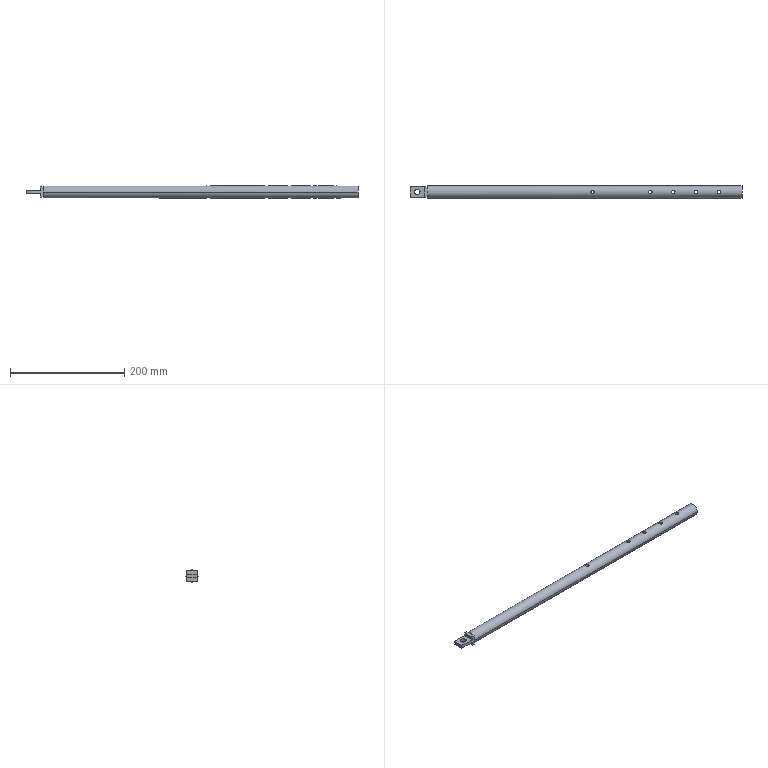Part | SolidWorks | features ICE 4, Revolution 1 | 1 solid | 32 faces | box 580 x 21 x 21 mm | volume 191345 mm3 | plane 18 | cylinder 14 | commonest cylinder face diameters 6 x10 10 x2 21 x2